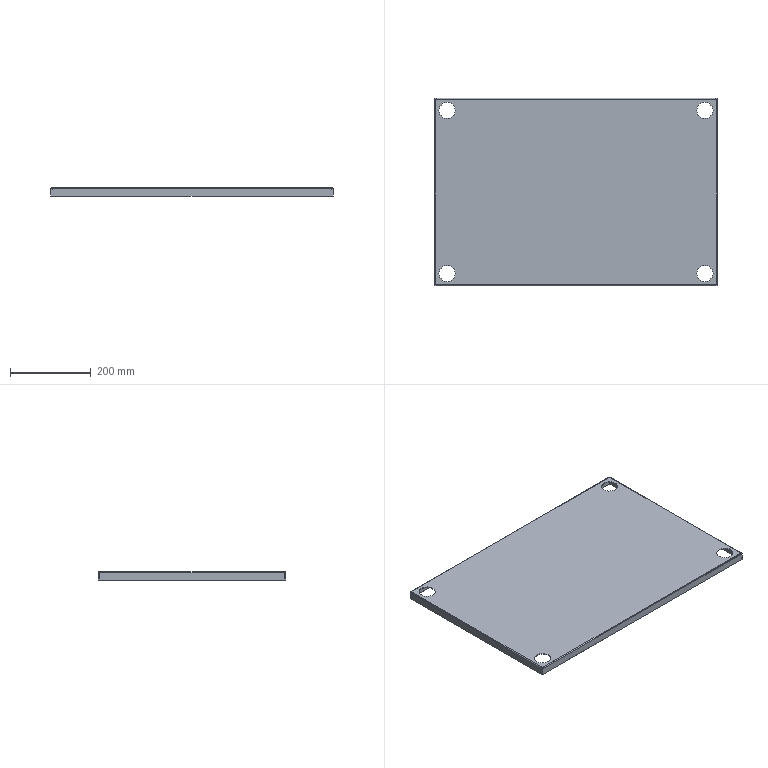Part | SolidWorks | features Extrusion 1, FlatPattern 1, FlattenBends 1, ICE 1, ProcessBends 1, Rip 1, SheetMetal 1, Shell 1 | 1 solid | 66 faces | box 697 x 463 x 20 mm | volume 716512 mm3 | plane 54 | cylinder 12 | commonest cylinder face diameters 40 x8 4 x4